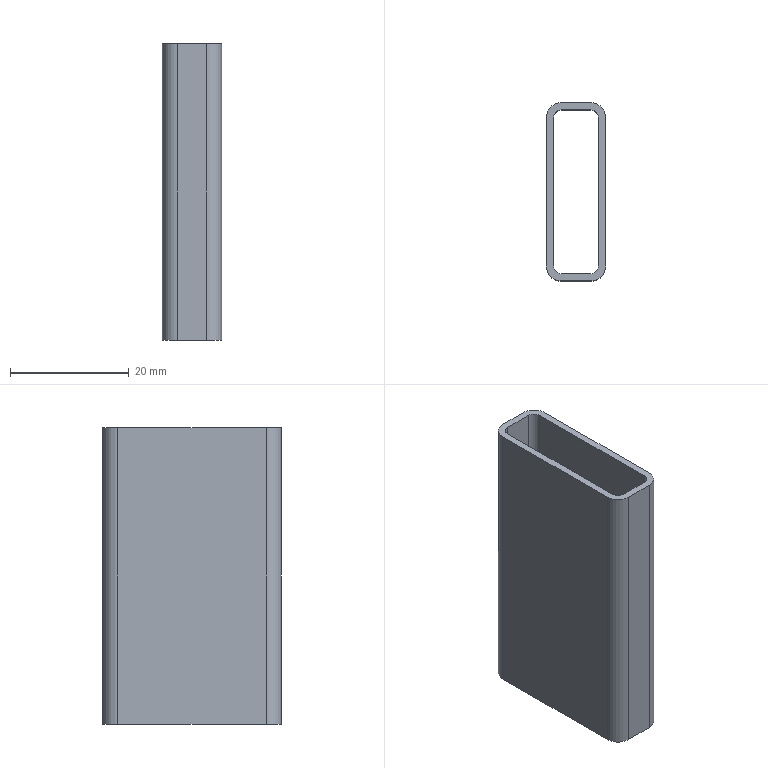Part | STEP file | 7100511 | 1 solid | 18 faces | box 10 x 30 x 50 mm | volume 4316 mm3 | plane 10 | cylinder 8 | commonest cylinder face diameters 2.6 x4 5 x4